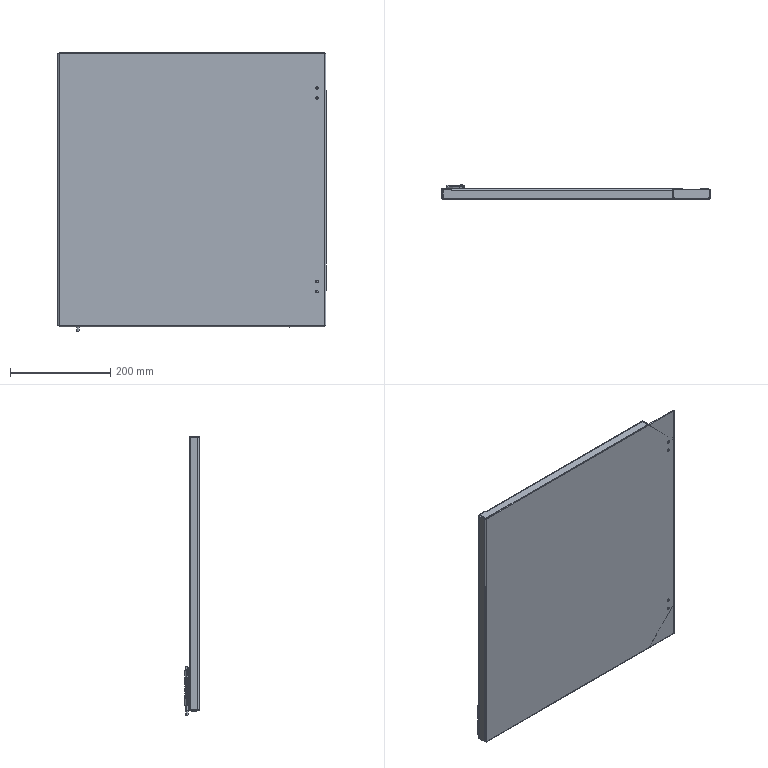Part | NX | features BREP 6 | 7 solids | 168 faces | box 534.5 x 29.2 x 557.003 mm | volume 549700 mm3 | plane 92 | cylinder 62 | torus 8 | spline 4 | cone 2 | commonest cylinder face diameters 6 x16 3 x8 5 x8 10 x8 0.8 x7 4 x6